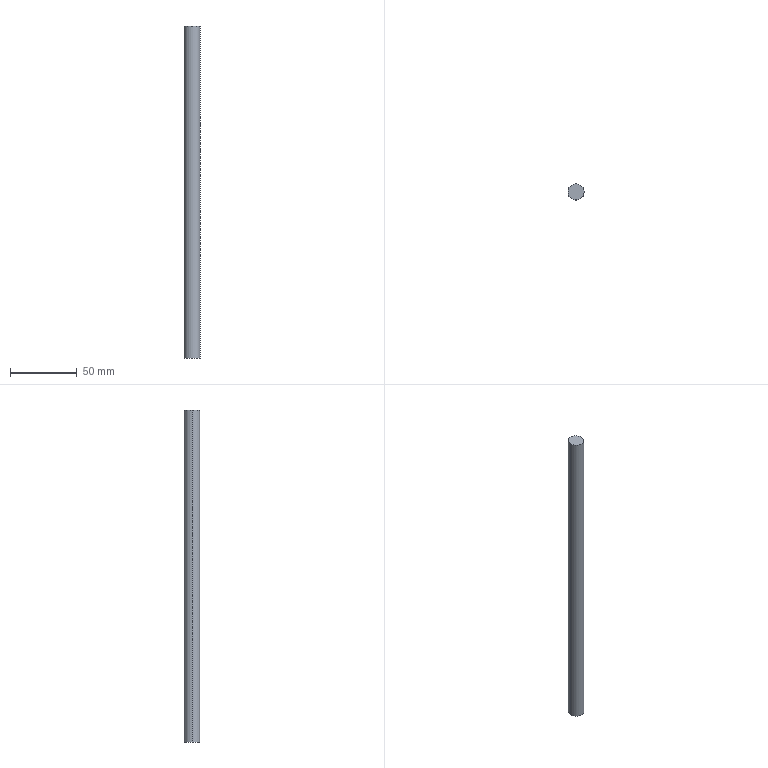Part | SolidWorks | features Extrusion 1 | 1 solid | 4 faces | box 12 x 12 x 249 mm | volume 28161 mm3 | cylinder 2 | plane 2 | commonest cylinder face diameters 12 x2
STEP:
#1=CARTESIAN_POINT('',(6.,0.,124.5));
#2=VERTEX_POINT('',#1);
#3=CARTESIAN_POINT('',(-6.,0.,124.5));
#4=VERTEX_POINT('',#3);
#5=CARTESIAN_POINT('',(0.,0.,124.5));
#6=DIRECTION('',(0.,0.,1.));
#7=DIRECTION('',(1.,0.,0.));
#8=AXIS2_PLACEMENT_3D('',#5,#6,#7);
#9=CIRCLE('',#8,6.);
#10=EDGE_CURVE('',#2,#4,#9,.T.);
#11=ORIENTED_EDGE('',*,*,#10,.F.);
#12=CARTESIAN_POINT('',(6.,0.,-124.5));
#13=VERTEX_POINT('',#12);
#14=CARTESIAN_POINT('',(6.,0.,124.5));
#15=DIRECTION('',(0.,0.,-1.));
#16=VECTOR('',#15,1000.);
#17=LINE('',#14,#16);
#18=EDGE_CURVE('',#2,#13,#17,.T.);
#19=ORIENTED_EDGE('',*,*,#18,.T.);
#20=CARTESIAN_POINT('',(-6.,0.,-124.5));
#21=VERTEX_POINT('',#20);
#22=CARTESIAN_POINT('',(0.,0.,-124.5));
#23=DIRECTION('',(0.,0.,1.));
#24=DIRECTION('',(1.,0.,0.));
#25=AXIS2_PLACEMENT_3D('',#22,#23,#24);
#26=CIRCLE('',#25,6.);
#27=EDGE_CURVE('',#13,#21,#26,.T.);
#28=ORIENTED_EDGE('',*,*,#27,.T.);
#29=CARTESIAN_POINT('',(-6.,0.,124.5));
#30=DIRECTION('',(0.,0.,-1.));
#31=VECTOR('',#30,1000.);
#32=LINE('',#29,#31);
#33=EDGE_CURVE('',#4,#21,#32,.T.);
#34=ORIENTED_EDGE('',*,*,#33,.F.);
#35=EDGE_LOOP('',(#11,#19,#28,#34));
#36=FACE_OUTER_BOUND('',#35,.T.);
#37=CARTESIAN_POINT('',(0.,0.,124.5));
#38=DIRECTION('',(0.,0.,-1.));
#39=DIRECTION('',(-1.,0.,0.));
#40=AXIS2_PLACEMENT_3D('',#37,#38,#39);
#41=CYLINDRICAL_SURFACE('',#40,6.);
#42=ADVANCED_FACE('',(#36),#41,.T.);
#43=ORIENTED_EDGE('',*,*,#18,.F.);
#44=CARTESIAN_POINT('',(0.,0.,124.5));
#45=DIRECTION('',(0.,0.,1.));
#46=DIRECTION('',(1.,0.,0.));
#47=AXIS2_PLACEMENT_3D('',#44,#45,#46);
#48=CIRCLE('',#47,6.);
#49=EDGE_CURVE('',#4,#2,#48,.T.);
#50=ORIENTED_EDGE('',*,*,#49,.F.);
#51=ORIENTED_EDGE('',*,*,#33,.T.);
#52=CARTESIAN_POINT('',(0.,0.,-124.5));
#53=DIRECTION('',(0.,0.,1.));
#54=DIRECTION('',(1.,0.,0.));
#55=AXIS2_PLACEMENT_3D('',#52,#53,#54);
#56=CIRCLE('',#55,6.);
#57=EDGE_CURVE('',#21,#13,#56,.T.);
#58=ORIENTED_EDGE('',*,*,#57,.T.);
#59=EDGE_LOOP('',(#43,#50,#51,#58));
#60=FACE_OUTER_BOUND('',#59,.T.);
#61=CARTESIAN_POINT('',(0.,0.,124.5));
#62=DIRECTION('',(0.,0.,-1.));
#63=DIRECTION('',(-1.,0.,0.));
#64=AXIS2_PLACEMENT_3D('',#61,#62,#63);
#65=CYLINDRICAL_SURFACE('',#64,6.);
#66=ADVANCED_FACE('',(#60),#65,.T.);
#67=ORIENTED_EDGE('',*,*,#49,.T.);
#68=ORIENTED_EDGE('',*,*,#10,.T.);
#69=EDGE_LOOP('',(#67,#68));
#70=FACE_OUTER_BOUND('',#69,.T.);
#71=CARTESIAN_POINT('',(0.,0.,124.5));
#72=DIRECTION('',(0.,0.,1.));
#73=DIRECTION('',(1.,0.,0.));
#74=AXIS2_PLACEMENT_3D('',#71,#72,#73);
#75=PLANE('',#74);
#76=ADVANCED_FACE('',(#70),#75,.T.);
#77=ORIENTED_EDGE('',*,*,#57,.F.);
#78=ORIENTED_EDGE('',*,*,#27,.F.);
#79=EDGE_LOOP('',(#77,#78));
#80=FACE_OUTER_BOUND('',#79,.T.);
#81=CARTESIAN_POINT('',(0.,0.,-124.5));
#82=DIRECTION('',(0.,0.,1.));
#83=DIRECTION('',(1.,0.,0.));
#84=AXIS2_PLACEMENT_3D('',#81,#82,#83);
#85=PLANE('',#84);
#86=ADVANCED_FACE('',(#80),#85,.F.);
#87=CLOSED_SHELL('',(#42,#66,#76,#86));
#88=MANIFOLD_SOLID_BREP('',#87);
#89=CARTESIAN_POINT('',(0.,0.,0.));
#90=DIRECTION('',(0.,0.,1.));
#91=DIRECTION('',(1.,0.,0.));
#92=AXIS2_PLACEMENT_3D('',#89,#90,#91);
#93=(LENGTH_UNIT()NAMED_UNIT(*)SI_UNIT(.MILLI.,.METRE.));
#94=UNCERTAINTY_MEASURE_WITH_UNIT(LENGTH_MEASURE(0.00001),#93,'','');
#95=(NAMED_UNIT(*)PLANE_ANGLE_UNIT()SI_UNIT($,.RADIAN.));
#96=(NAMED_UNIT(*)SI_UNIT($,.STERADIAN.)SOLID_ANGLE_UNIT());
#97=(GEOMETRIC_REPRESENTATION_CONTEXT(3)GLOBAL_UNCERTAINTY_ASSIGNED_CONTEXT((#94))GLOBAL_UNIT_ASSIGNED_CONTEXT((#93,#95,#96))REPRESENTATION_CONTEXT('',''));
#98=ADVANCED_BREP_SHAPE_REPRESENTATION('',(#88,#92),#97);